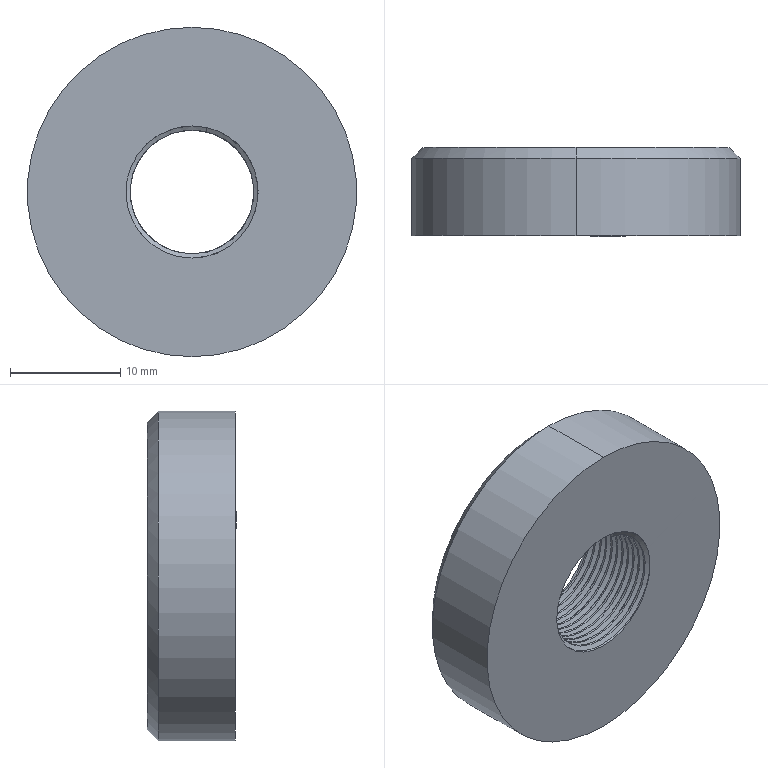Part | SolidWorks | features Chamfer 1, Extrusion 1, SweepThread 1 | 1 solid | 36 faces | box 29.9 x 8.112 x 29.9 mm | volume 4725 mm3 | cylinder 26 | plane 4 | spline 4 | cone 2 | commonest cylinder face diameters 12 x24 29.9 x2